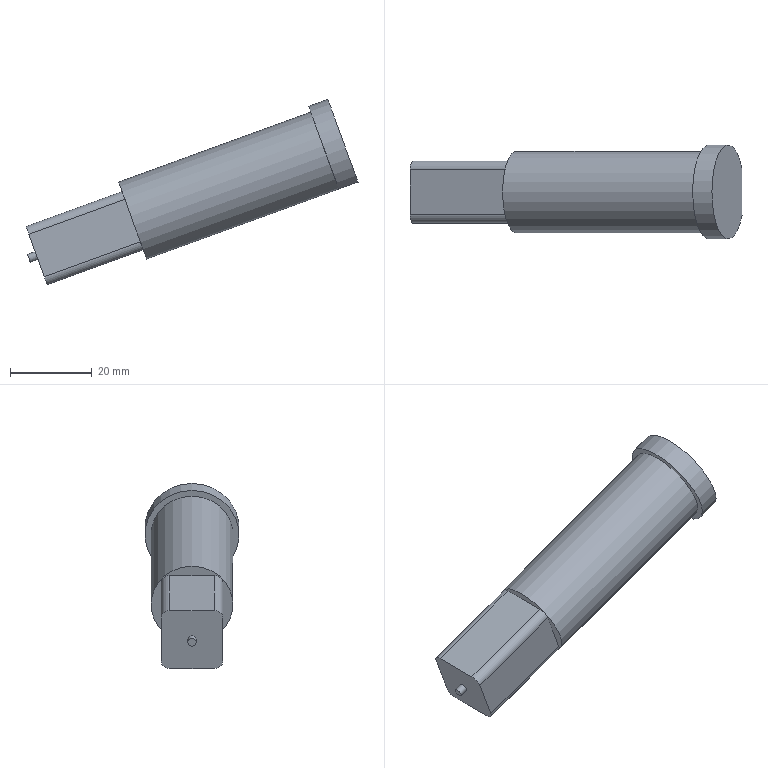Part | NX | features solid 2 | 1 solid | 17 faces | box 81.178 x 23 x 45.263 mm | volume 23344 mm3 | plane 10 | cylinder 7 | commonest cylinder face diameters 4.1 x4 2 x1 20 x1 23 x1
STEP:
#1=CARTESIAN_POINT('',(683.044,-286.995,42.482));
#2=VERTEX_POINT('',#1);
#3=CARTESIAN_POINT('',(686.464,-286.994,33.085));
#4=DIRECTION('',(-0.9397,0.000001517,-0.342));
#5=DIRECTION('',(-0.342,-0.0001374,0.9397));
#6=AXIS2_PLACEMENT_3D('',#3,#4,#5);
#7=CIRCLE('',#6,10.);
#8=EDGE_CURVE('',#2,#2,#7,.T.);
#9=ORIENTED_EDGE('',*,*,#8,.T.);
#10=EDGE_LOOP('',(#9));
#11=FACE_BOUND('',#10,.T.);
#12=CARTESIAN_POINT('',(689.046,-281.493,25.991));
#13=VERTEX_POINT('',#12);
#14=CARTESIAN_POINT('',(689.047,-292.493,25.99));
#15=VERTEX_POINT('',#14);
#16=CARTESIAN_POINT('',(689.046,-279.443,25.992));
#17=DIRECTION('',(0.00004556,-1.,-0.0001296));
#18=VECTOR('',#17,1000.);
#19=LINE('',#16,#18);
#20=EDGE_CURVE('',#13,#15,#19,.T.);
#21=ORIENTED_EDGE('',*,*,#20,.F.);
#22=CARTESIAN_POINT('',(688.345,-279.443,27.918));
#23=VERTEX_POINT('',#22);
#24=CARTESIAN_POINT('',(688.345,-281.493,27.918));
#25=DIRECTION('',(-0.9397,0.000001517,-0.342));
#26=DIRECTION('',(-0.342,-0.0001374,0.9397));
#27=AXIS2_PLACEMENT_3D('',#24,#25,#26);
#28=CIRCLE('',#27,2.05);
#29=EDGE_CURVE('',#23,#13,#28,.T.);
#30=ORIENTED_EDGE('',*,*,#29,.F.);
#31=CARTESIAN_POINT('',(684.583,-279.445,38.255));
#32=VERTEX_POINT('',#31);
#33=CARTESIAN_POINT('',(683.881,-279.445,40.181));
#34=DIRECTION('',(0.342,0.0001374,-0.9397));
#35=VECTOR('',#34,1000.);
#36=LINE('',#33,#35);
#37=EDGE_CURVE('',#32,#23,#36,.T.);
#38=ORIENTED_EDGE('',*,*,#37,.F.);
#39=CARTESIAN_POINT('',(683.882,-281.495,40.181));
#40=VERTEX_POINT('',#39);
#41=CARTESIAN_POINT('',(684.583,-281.495,38.254));
#42=DIRECTION('',(-0.9397,0.000001517,-0.342));
#43=DIRECTION('',(-0.342,-0.0001374,0.9397));
#44=AXIS2_PLACEMENT_3D('',#41,#42,#43);
#45=CIRCLE('',#44,2.05);
#46=EDGE_CURVE('',#40,#32,#45,.T.);
#47=ORIENTED_EDGE('',*,*,#46,.F.);
#48=CARTESIAN_POINT('',(683.882,-292.495,40.179));
#49=VERTEX_POINT('',#48);
#50=CARTESIAN_POINT('',(683.881,-279.445,40.181));
#51=DIRECTION('',(0.00004556,-1.,-0.0001296));
#52=VECTOR('',#51,1000.);
#53=LINE('',#50,#52);
#54=EDGE_CURVE('',#40,#49,#53,.T.);
#55=ORIENTED_EDGE('',*,*,#54,.T.);
#56=CARTESIAN_POINT('',(684.583,-294.545,38.253));
#57=VERTEX_POINT('',#56);
#58=CARTESIAN_POINT('',(684.583,-292.495,38.253));
#59=DIRECTION('',(-0.9397,0.000001517,-0.342));
#60=DIRECTION('',(-0.342,-0.0001374,0.9397));
#61=AXIS2_PLACEMENT_3D('',#58,#59,#60);
#62=CIRCLE('',#61,2.05);
#63=EDGE_CURVE('',#57,#49,#62,.T.);
#64=ORIENTED_EDGE('',*,*,#63,.F.);
#65=CARTESIAN_POINT('',(688.345,-294.543,27.916));
#66=VERTEX_POINT('',#65);
#67=CARTESIAN_POINT('',(689.047,-294.543,25.99));
#68=DIRECTION('',(-0.342,-0.0001374,0.9397));
#69=VECTOR('',#68,1000.);
#70=LINE('',#67,#69);
#71=EDGE_CURVE('',#66,#57,#70,.T.);
#72=ORIENTED_EDGE('',*,*,#71,.F.);
#73=CARTESIAN_POINT('',(688.345,-292.493,27.916));
#74=DIRECTION('',(-0.9397,0.000001517,-0.342));
#75=DIRECTION('',(-0.342,-0.0001374,0.9397));
#76=AXIS2_PLACEMENT_3D('',#73,#74,#75);
#77=CIRCLE('',#76,2.05);
#78=EDGE_CURVE('',#15,#66,#77,.T.);
#79=ORIENTED_EDGE('',*,*,#78,.F.);
#80=EDGE_LOOP('',(#21,#30,#38,#47,#55,#64,#72,#79));
#81=FACE_BOUND('',#80,.T.);
#82=CARTESIAN_POINT('',(686.464,-286.994,33.085));
#83=DIRECTION('',(0.9397,-0.000001517,0.342));
#84=DIRECTION('',(-0.342,-0.0001374,0.9397));
#85=AXIS2_PLACEMENT_3D('',#82,#83,#84);
#86=PLANE('',#85);
#87=ADVANCED_FACE('',(#11,#81),#86,.F.);
#88=ORIENTED_EDGE('',*,*,#8,.F.);
#89=EDGE_LOOP('',(#88));
#90=FACE_BOUND('',#89,.T.);
#91=CARTESIAN_POINT('',(736.869,-286.993,40.789));
#92=VERTEX_POINT('',#91);
#93=CARTESIAN_POINT('',(733.449,-286.994,50.186));
#94=DIRECTION('',(-0.9397,0.000001517,-0.342));
#95=DIRECTION('',(-0.342,-0.0001374,0.9397));
#96=AXIS2_PLACEMENT_3D('',#93,#94,#95);
#97=CIRCLE('',#96,10.);
#98=EDGE_CURVE('',#92,#92,#97,.T.);
#99=ORIENTED_EDGE('',*,*,#98,.T.);
#100=EDGE_LOOP('',(#99));
#101=FACE_BOUND('',#100,.T.);
#102=CARTESIAN_POINT('',(738.147,-286.994,51.896));
#103=DIRECTION('',(-0.9397,0.000001517,-0.342));
#104=DIRECTION('',(0.342,0.0001374,-0.9397));
#105=AXIS2_PLACEMENT_3D('',#102,#103,#104);
#106=CYLINDRICAL_SURFACE('',#105,10.);
#107=ADVANCED_FACE('',(#90,#101),#106,.T.);
#108=CARTESIAN_POINT('',(736.869,-292.672,40.789));
#109=VERTEX_POINT('',#108);
#110=CARTESIAN_POINT('',(736.869,-281.314,40.79));
#111=VERTEX_POINT('',#110);
#112=CARTESIAN_POINT('',(733.449,-286.994,50.186));
#113=DIRECTION('',(-0.9397,0.000001517,-0.342));
#114=DIRECTION('',(-0.342,-0.0001374,0.9397));
#115=AXIS2_PLACEMENT_3D('',#112,#113,#114);
#116=CIRCLE('',#115,11.5);
#117=EDGE_CURVE('',#109,#111,#116,.T.);
#118=ORIENTED_EDGE('',*,*,#117,.T.);
#119=CARTESIAN_POINT('',(736.869,-286.993,40.789));
#120=DIRECTION('',(-0.00004556,1.,0.0001296));
#121=VECTOR('',#120,1000.);
#122=LINE('',#119,#121);
#123=EDGE_CURVE('',#92,#111,#122,.T.);
#124=ORIENTED_EDGE('',*,*,#123,.F.);
#125=ORIENTED_EDGE('',*,*,#98,.F.);
#126=CARTESIAN_POINT('',(736.869,-286.993,40.789));
#127=DIRECTION('',(-0.00004556,1.,0.0001296));
#128=VECTOR('',#127,1000.);
#129=LINE('',#126,#128);
#130=EDGE_CURVE('',#109,#92,#129,.T.);
#131=ORIENTED_EDGE('',*,*,#130,.F.);
#132=EDGE_LOOP('',(#118,#124,#125,#131));
#133=FACE_BOUND('',#132,.T.);
#134=CARTESIAN_POINT('',(733.449,-286.994,50.186));
#135=DIRECTION('',(0.9397,-0.000001517,0.342));
#136=DIRECTION('',(-0.342,-0.0001374,0.9397));
#137=AXIS2_PLACEMENT_3D('',#134,#135,#136);
#138=PLANE('',#137);
#139=ADVANCED_FACE('',(#133),#138,.F.);
#140=CARTESIAN_POINT('',(741.567,-281.314,42.5));
#141=VERTEX_POINT('',#140);
#142=CARTESIAN_POINT('',(744.386,-281.314,43.526));
#143=DIRECTION('',(-0.9397,0.000001517,-0.342));
#144=VECTOR('',#143,1000.);
#145=LINE('',#142,#144);
#146=EDGE_CURVE('',#111,#141,#145,.F.);
#147=ORIENTED_EDGE('',*,*,#146,.F.);
#148=ORIENTED_EDGE('',*,*,#117,.F.);
#149=CARTESIAN_POINT('',(741.568,-292.672,42.499));
#150=VERTEX_POINT('',#149);
#151=CARTESIAN_POINT('',(744.387,-292.672,43.525));
#152=DIRECTION('',(-0.9397,0.000001517,-0.342));
#153=VECTOR('',#152,1000.);
#154=LINE('',#151,#153);
#155=EDGE_CURVE('',#150,#109,#154,.T.);
#156=ORIENTED_EDGE('',*,*,#155,.F.);
#157=CARTESIAN_POINT('',(738.147,-286.994,51.896));
#158=DIRECTION('',(-0.9397,0.000001517,-0.342));
#159=DIRECTION('',(-0.342,-0.0001374,0.9397));
#160=AXIS2_PLACEMENT_3D('',#157,#158,#159);
#161=CIRCLE('',#160,11.5);
#162=EDGE_CURVE('',#150,#141,#161,.T.);
#163=ORIENTED_EDGE('',*,*,#162,.T.);
#164=EDGE_LOOP('',(#147,#148,#156,#163));
#165=FACE_BOUND('',#164,.T.);
#166=CARTESIAN_POINT('',(733.449,-286.994,50.186));
#167=DIRECTION('',(0.9397,-0.000001517,0.342));
#168=DIRECTION('',(-0.342,-0.0001374,0.9397));
#169=AXIS2_PLACEMENT_3D('',#166,#167,#168);
#170=CYLINDRICAL_SURFACE('',#169,11.5);
#171=ADVANCED_FACE('',(#165),#170,.T.);
#172=CARTESIAN_POINT('',(741.567,-286.993,42.5));
#173=DIRECTION('',(-0.00004556,1.,0.0001296));
#174=VECTOR('',#173,1000.);
#175=LINE('',#172,#174);
#176=EDGE_CURVE('',#150,#141,#175,.T.);
#177=ORIENTED_EDGE('',*,*,#176,.T.);
#178=ORIENTED_EDGE('',*,*,#162,.F.);
#179=EDGE_LOOP('',(#177,#178));
#180=FACE_BOUND('',#179,.T.);
#181=CARTESIAN_POINT('',(738.147,-286.994,51.896));
#182=DIRECTION('',(0.9397,-0.000001517,0.342));
#183=DIRECTION('',(-0.342,-0.0001374,0.9397));
#184=AXIS2_PLACEMENT_3D('',#181,#182,#183);
#185=PLANE('',#184);
#186=ADVANCED_FACE('',(#180),#185,.T.);
#187=ORIENTED_EDGE('',*,*,#155,.T.);
#188=ORIENTED_EDGE('',*,*,#130,.T.);
#189=ORIENTED_EDGE('',*,*,#123,.T.);
#190=ORIENTED_EDGE('',*,*,#146,.T.);
#191=ORIENTED_EDGE('',*,*,#176,.F.);
#192=EDGE_LOOP('',(#187,#188,#189,#190,#191));
#193=FACE_BOUND('',#192,.T.);
#194=CARTESIAN_POINT('',(744.386,-281.314,43.526));
#195=DIRECTION('',(-0.342,-0.0001374,0.9397));
#196=DIRECTION('',(-0.9397,0.000001517,-0.342));
#197=AXIS2_PLACEMENT_3D('',#194,#195,#196);
#198=PLANE('',#197);
#199=ADVANCED_FACE('',(#193),#198,.F.);
#200=CARTESIAN_POINT('',(664.853,-294.543,19.366));
#201=VERTEX_POINT('',#200);
#202=CARTESIAN_POINT('',(661.091,-294.545,29.702));
#203=VERTEX_POINT('',#202);
#204=CARTESIAN_POINT('',(665.554,-294.543,17.439));
#205=DIRECTION('',(-0.342,-0.0001374,0.9397));
#206=VECTOR('',#205,1000.);
#207=LINE('',#204,#206);
#208=EDGE_CURVE('',#201,#203,#207,.T.);
#209=ORIENTED_EDGE('',*,*,#208,.F.);
#210=CARTESIAN_POINT('',(664.853,-294.543,19.366));
#211=DIRECTION('',(0.9397,-0.000001517,0.342));
#212=VECTOR('',#211,1000.);
#213=LINE('',#210,#212);
#214=EDGE_CURVE('',#66,#201,#213,.F.);
#215=ORIENTED_EDGE('',*,*,#214,.F.);
#216=ORIENTED_EDGE('',*,*,#71,.T.);
#217=CARTESIAN_POINT('',(684.583,-294.545,38.253));
#218=DIRECTION('',(0.9397,-0.000001517,0.342));
#219=VECTOR('',#218,1000.);
#220=LINE('',#217,#219);
#221=EDGE_CURVE('',#203,#57,#220,.T.);
#222=ORIENTED_EDGE('',*,*,#221,.F.);
#223=EDGE_LOOP('',(#209,#215,#216,#222));
#224=FACE_BOUND('',#223,.T.);
#225=CARTESIAN_POINT('',(665.554,-294.543,17.439));
#226=DIRECTION('',(0.00004556,-1.,-0.0001296));
#227=DIRECTION('',(-0.9397,0.000001517,-0.342));
#228=AXIS2_PLACEMENT_3D('',#225,#226,#227);
#229=PLANE('',#228);
#230=ADVANCED_FACE('',(#224),#229,.T.);
#231=CARTESIAN_POINT('',(660.389,-281.495,31.63));
#232=VERTEX_POINT('',#231);
#233=CARTESIAN_POINT('',(660.39,-292.495,31.629));
#234=VERTEX_POINT('',#233);
#235=CARTESIAN_POINT('',(660.389,-279.445,31.631));
#236=DIRECTION('',(0.00004556,-1.,-0.0001296));
#237=VECTOR('',#236,1000.);
#238=LINE('',#235,#237);
#239=EDGE_CURVE('',#232,#234,#238,.T.);
#240=ORIENTED_EDGE('',*,*,#239,.T.);
#241=CARTESIAN_POINT('',(660.39,-292.495,31.629));
#242=DIRECTION('',(0.9397,-0.000001517,0.342));
#243=VECTOR('',#242,1000.);
#244=LINE('',#241,#243);
#245=EDGE_CURVE('',#49,#234,#244,.F.);
#246=ORIENTED_EDGE('',*,*,#245,.F.);
#247=ORIENTED_EDGE('',*,*,#54,.F.);
#248=CARTESIAN_POINT('',(683.882,-281.495,40.181));
#249=DIRECTION('',(0.9397,-0.000001517,0.342));
#250=VECTOR('',#249,1000.);
#251=LINE('',#248,#250);
#252=EDGE_CURVE('',#232,#40,#251,.T.);
#253=ORIENTED_EDGE('',*,*,#252,.F.);
#254=EDGE_LOOP('',(#240,#246,#247,#253));
#255=FACE_BOUND('',#254,.T.);
#256=CARTESIAN_POINT('',(660.389,-279.445,31.631));
#257=DIRECTION('',(0.342,0.0001374,-0.9397));
#258=DIRECTION('',(0.9397,-0.000001517,0.342));
#259=AXIS2_PLACEMENT_3D('',#256,#257,#258);
#260=PLANE('',#259);
#261=ADVANCED_FACE('',(#255),#260,.F.);
#262=ORIENTED_EDGE('',*,*,#37,.T.);
#263=CARTESIAN_POINT('',(664.852,-279.443,19.368));
#264=VERTEX_POINT('',#263);
#265=CARTESIAN_POINT('',(664.852,-279.443,19.368));
#266=DIRECTION('',(0.9397,-0.000001517,0.342));
#267=VECTOR('',#266,1000.);
#268=LINE('',#265,#267);
#269=EDGE_CURVE('',#264,#23,#268,.T.);
#270=ORIENTED_EDGE('',*,*,#269,.F.);
#271=CARTESIAN_POINT('',(661.09,-279.445,29.704));
#272=VERTEX_POINT('',#271);
#273=CARTESIAN_POINT('',(660.389,-279.445,31.631));
#274=DIRECTION('',(0.342,0.0001374,-0.9397));
#275=VECTOR('',#274,1000.);
#276=LINE('',#273,#275);
#277=EDGE_CURVE('',#272,#264,#276,.T.);
#278=ORIENTED_EDGE('',*,*,#277,.F.);
#279=CARTESIAN_POINT('',(661.09,-279.445,29.704));
#280=DIRECTION('',(0.9397,-0.000001517,0.342));
#281=VECTOR('',#280,1000.);
#282=LINE('',#279,#281);
#283=EDGE_CURVE('',#32,#272,#282,.F.);
#284=ORIENTED_EDGE('',*,*,#283,.F.);
#285=EDGE_LOOP('',(#262,#270,#278,#284));
#286=FACE_BOUND('',#285,.T.);
#287=CARTESIAN_POINT('',(660.389,-279.445,31.631));
#288=DIRECTION('',(-0.00004556,1.,0.0001296));
#289=DIRECTION('',(0.9397,-0.000001517,0.342));
#290=AXIS2_PLACEMENT_3D('',#287,#288,#289);
#291=PLANE('',#290);
#292=ADVANCED_FACE('',(#286),#291,.T.);
#293=ORIENTED_EDGE('',*,*,#20,.T.);
#294=CARTESIAN_POINT('',(665.554,-292.493,17.44));
#295=VERTEX_POINT('',#294);
#296=CARTESIAN_POINT('',(665.554,-292.493,17.44));
#297=DIRECTION('',(0.9397,-0.000001517,0.342));
#298=VECTOR('',#297,1000.);
#299=LINE('',#296,#298);
#300=EDGE_CURVE('',#295,#15,#299,.T.);
#301=ORIENTED_EDGE('',*,*,#300,.F.);
#302=CARTESIAN_POINT('',(665.554,-281.493,17.441));
#303=VERTEX_POINT('',#302);
#304=CARTESIAN_POINT('',(665.554,-279.443,17.441));
#305=DIRECTION('',(0.00004556,-1.,-0.0001296));
#306=VECTOR('',#305,1000.);
#307=LINE('',#304,#306);
#308=EDGE_CURVE('',#303,#295,#307,.T.);
#309=ORIENTED_EDGE('',*,*,#308,.F.);
#310=CARTESIAN_POINT('',(665.554,-281.493,17.441));
#311=DIRECTION('',(0.9397,-0.000001517,0.342));
#312=VECTOR('',#311,1000.);
#313=LINE('',#310,#312);
#314=EDGE_CURVE('',#13,#303,#313,.F.);
#315=ORIENTED_EDGE('',*,*,#314,.F.);
#316=EDGE_LOOP('',(#293,#301,#309,#315));
#317=FACE_BOUND('',#316,.T.);
#318=CARTESIAN_POINT('',(665.554,-279.443,17.441));
#319=DIRECTION('',(0.342,0.0001374,-0.9397));
#320=DIRECTION('',(0.9397,-0.000001517,0.342));
#321=AXIS2_PLACEMENT_3D('',#318,#319,#320);
#322=PLANE('',#321);
#323=ADVANCED_FACE('',(#317),#322,.T.);
#324=CARTESIAN_POINT('',(663.314,-286.994,23.595));
#325=VERTEX_POINT('',#324);
#326=CARTESIAN_POINT('',(662.972,-286.994,24.535));
#327=DIRECTION('',(0.9397,-0.000001517,0.342));
#328=DIRECTION('',(0.342,0.0001374,-0.9397));
#329=AXIS2_PLACEMENT_3D('',#326,#327,#328);
#330=CIRCLE('',#329,1.);
#331=EDGE_CURVE('',#325,#325,#330,.T.);
#332=ORIENTED_EDGE('',*,*,#331,.T.);
#333=EDGE_LOOP('',(#332));
#334=FACE_BOUND('',#333,.T.);
#335=ORIENTED_EDGE('',*,*,#277,.T.);
#336=CARTESIAN_POINT('',(664.853,-281.493,19.367));
#337=DIRECTION('',(0.9397,-0.000001517,0.342));
#338=DIRECTION('',(0.342,0.0001374,-0.9397));
#339=AXIS2_PLACEMENT_3D('',#336,#337,#338);
#340=CIRCLE('',#339,2.05);
#341=EDGE_CURVE('',#303,#264,#340,.T.);
#342=ORIENTED_EDGE('',*,*,#341,.F.);
#343=ORIENTED_EDGE('',*,*,#308,.T.);
#344=CARTESIAN_POINT('',(664.853,-292.493,19.366));
#345=DIRECTION('',(0.9397,-0.000001517,0.342));
#346=DIRECTION('',(0.342,0.0001374,-0.9397));
#347=AXIS2_PLACEMENT_3D('',#344,#345,#346);
#348=CIRCLE('',#347,2.05);
#349=EDGE_CURVE('',#201,#295,#348,.T.);
#350=ORIENTED_EDGE('',*,*,#349,.F.);
#351=ORIENTED_EDGE('',*,*,#208,.T.);
#352=CARTESIAN_POINT('',(661.091,-292.495,29.702));
#353=DIRECTION('',(0.9397,-0.000001517,0.342));
#354=DIRECTION('',(0.342,0.0001374,-0.9397));
#355=AXIS2_PLACEMENT_3D('',#352,#353,#354);
#356=CIRCLE('',#355,2.05);
#357=EDGE_CURVE('',#234,#203,#356,.T.);
#358=ORIENTED_EDGE('',*,*,#357,.F.);
#359=ORIENTED_EDGE('',*,*,#239,.F.);
#360=CARTESIAN_POINT('',(661.09,-281.495,29.704));
#361=DIRECTION('',(0.9397,-0.000001517,0.342));
#362=DIRECTION('',(0.342,0.0001374,-0.9397));
#363=AXIS2_PLACEMENT_3D('',#360,#361,#362);
#364=CIRCLE('',#363,2.05);
#365=EDGE_CURVE('',#272,#232,#364,.T.);
#366=ORIENTED_EDGE('',*,*,#365,.F.);
#367=EDGE_LOOP('',(#335,#342,#343,#350,#351,#358,#359,#366));
#368=FACE_BOUND('',#367,.T.);
#369=CARTESIAN_POINT('',(660.39,-294.545,31.629));
#370=DIRECTION('',(-0.9397,0.000001517,-0.342));
#371=DIRECTION('',(0.342,0.0001374,-0.9397));
#372=AXIS2_PLACEMENT_3D('',#369,#370,#371);
#373=PLANE('',#372);
#374=ADVANCED_FACE('',(#334,#368),#373,.T.);
#375=ORIENTED_EDGE('',*,*,#365,.T.);
#376=ORIENTED_EDGE('',*,*,#252,.T.);
#377=ORIENTED_EDGE('',*,*,#46,.T.);
#378=ORIENTED_EDGE('',*,*,#283,.T.);
#379=EDGE_LOOP('',(#375,#376,#377,#378));
#380=FACE_BOUND('',#379,.T.);
#381=CARTESIAN_POINT('',(661.09,-281.495,29.704));
#382=DIRECTION('',(-0.9397,0.000001517,-0.342));
#383=DIRECTION('',(0.342,0.0001374,-0.9397));
#384=AXIS2_PLACEMENT_3D('',#381,#382,#383);
#385=CYLINDRICAL_SURFACE('',#384,2.05);
#386=ADVANCED_FACE('',(#380),#385,.T.);
#387=ORIENTED_EDGE('',*,*,#341,.T.);
#388=ORIENTED_EDGE('',*,*,#269,.T.);
#389=ORIENTED_EDGE('',*,*,#29,.T.);
#390=ORIENTED_EDGE('',*,*,#314,.T.);
#391=EDGE_LOOP('',(#387,#388,#389,#390));
#392=FACE_BOUND('',#391,.T.);
#393=CARTESIAN_POINT('',(664.853,-281.493,19.367));
#394=DIRECTION('',(0.9397,-0.000001517,0.342));
#395=DIRECTION('',(-0.342,-0.0001374,0.9397));
#396=AXIS2_PLACEMENT_3D('',#393,#394,#395);
#397=CYLINDRICAL_SURFACE('',#396,2.05);
#398=ADVANCED_FACE('',(#392),#397,.T.);
#399=ORIENTED_EDGE('',*,*,#357,.T.);
#400=ORIENTED_EDGE('',*,*,#221,.T.);
#401=ORIENTED_EDGE('',*,*,#63,.T.);
#402=ORIENTED_EDGE('',*,*,#245,.T.);
#403=EDGE_LOOP('',(#399,#400,#401,#402));
#404=FACE_BOUND('',#403,.T.);
#405=CARTESIAN_POINT('',(661.091,-292.495,29.702));
#406=DIRECTION('',(-0.9397,0.000001517,-0.342));
#407=DIRECTION('',(0.342,0.0001374,-0.9397));
#408=AXIS2_PLACEMENT_3D('',#405,#406,#407);
#409=CYLINDRICAL_SURFACE('',#408,2.05);
#410=ADVANCED_FACE('',(#404),#409,.T.);
#411=ORIENTED_EDGE('',*,*,#349,.T.);
#412=ORIENTED_EDGE('',*,*,#300,.T.);
#413=ORIENTED_EDGE('',*,*,#78,.T.);
#414=ORIENTED_EDGE('',*,*,#214,.T.);
#415=EDGE_LOOP('',(#411,#412,#413,#414));
#416=FACE_BOUND('',#415,.T.);
#417=CARTESIAN_POINT('',(664.853,-292.493,19.366));
#418=DIRECTION('',(0.9397,-0.000001517,0.342));
#419=DIRECTION('',(-0.342,-0.0001374,0.9397));
#420=AXIS2_PLACEMENT_3D('',#417,#418,#419);
#421=CYLINDRICAL_SURFACE('',#420,2.05);
#422=ADVANCED_FACE('',(#416),#421,.T.);
#423=CARTESIAN_POINT('',(660.75,-286.994,24.791));
#424=VERTEX_POINT('',#423);
#425=CARTESIAN_POINT('',(661.092,-286.994,23.851));
#426=DIRECTION('',(-0.9397,0.000001517,-0.342));
#427=DIRECTION('',(-0.342,-0.0001374,0.9397));
#428=AXIS2_PLACEMENT_3D('',#425,#426,#427);
#429=CIRCLE('',#428,1.);
#430=EDGE_CURVE('',#424,#424,#429,.T.);
#431=ORIENTED_EDGE('',*,*,#430,.F.);
#432=EDGE_LOOP('',(#431));
#433=FACE_BOUND('',#432,.T.);
#434=ORIENTED_EDGE('',*,*,#331,.F.);
#435=EDGE_LOOP('',(#434));
#436=FACE_BOUND('',#435,.T.);
#437=CARTESIAN_POINT('',(661.092,-286.994,23.851));
#438=DIRECTION('',(0.9397,-0.000001517,0.342));
#439=DIRECTION('',(-0.342,-0.0001374,0.9397));
#440=AXIS2_PLACEMENT_3D('',#437,#438,#439);
#441=CYLINDRICAL_SURFACE('',#440,1.);
#442=ADVANCED_FACE('',(#433,#436),#441,.T.);
#443=ORIENTED_EDGE('',*,*,#430,.T.);
#444=EDGE_LOOP('',(#443));
#445=FACE_BOUND('',#444,.T.);
#446=CARTESIAN_POINT('',(661.092,-286.994,23.851));
#447=DIRECTION('',(0.9397,-0.000001517,0.342));
#448=DIRECTION('',(-0.342,-0.0001374,0.9397));
#449=AXIS2_PLACEMENT_3D('',#446,#447,#448);
#450=PLANE('',#449);
#451=ADVANCED_FACE('',(#445),#450,.F.);
#452=CLOSED_SHELL('',(#87,#107,#139,#171,#186,#199,#230,#261,#292,#323,#374,#386,#398,#410,#422,#442,#451));
#453=MANIFOLD_SOLID_BREP('',#452);
#454=(LENGTH_UNIT()NAMED_UNIT(*)SI_UNIT(.MILLI.,.METRE.));
#455=UNCERTAINTY_MEASURE_WITH_UNIT(LENGTH_MEASURE(0.00001),#454,'','');
#456=(NAMED_UNIT(*)PLANE_ANGLE_UNIT()SI_UNIT($,.RADIAN.));
#457=(NAMED_UNIT(*)SI_UNIT($,.STERADIAN.)SOLID_ANGLE_UNIT());
#458=(GEOMETRIC_REPRESENTATION_CONTEXT(3)GLOBAL_UNCERTAINTY_ASSIGNED_CONTEXT((#455))GLOBAL_UNIT_ASSIGNED_CONTEXT((#454,#456,#457))REPRESENTATION_CONTEXT('',''));
#459=ADVANCED_BREP_SHAPE_REPRESENTATION('',(#453),#458);